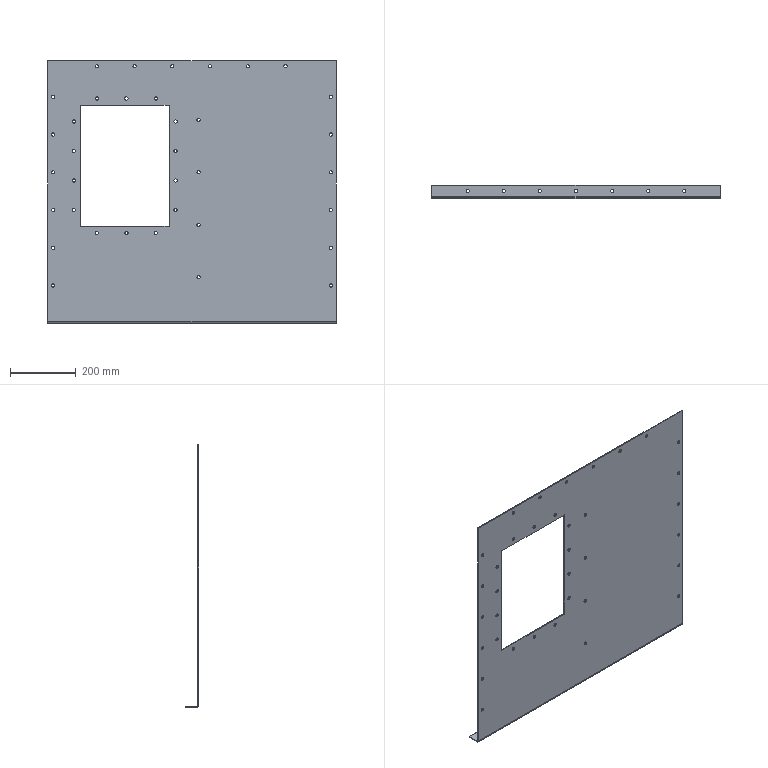Part | SolidWorks | features ICE 5, EdgeFlange 1, FlatPattern 1, SMBaseFlange 1, SheetMetal 1 | 1 solid | 104 faces | box 880 x 40 x 800 mm | volume 1894749 mm3 | cylinder 88 | plane 16 | commonest cylinder face diameters 10 x86 6 x1 12 x1